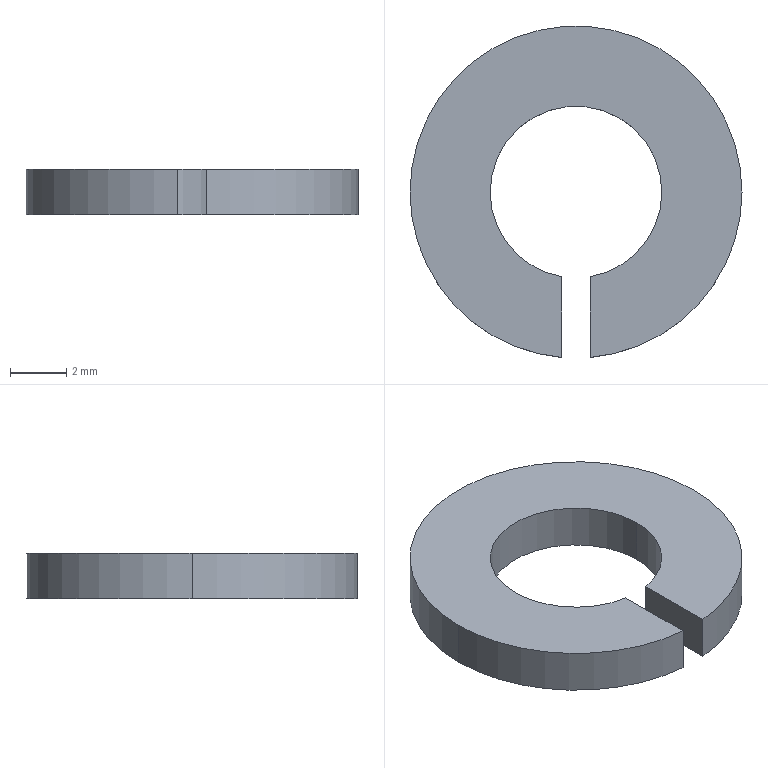Part | NX | features BREP 1 | 1 solid | 10 faces | box 11.8 x 11.779 x 1.6 mm | volume 123.644 mm3 | cylinder 6 | plane 4 | commonest cylinder face diameters 6.1 x3 11.8 x3
STEP:
#1=CARTESIAN_POINT('',(3.05,0.,1.6));
#2=VERTEX_POINT('',#1);
#3=CARTESIAN_POINT('',(0.5,-3.009,1.6));
#4=VERTEX_POINT('',#3);
#5=CARTESIAN_POINT('',(0.,0.,1.6));
#6=DIRECTION('',(0.,0.,-1.));
#7=DIRECTION('',(1.,0.,0.));
#8=AXIS2_PLACEMENT_3D('',#5,#6,#7);
#9=CIRCLE('',#8,3.05);
#10=EDGE_CURVE('',#2,#4,#9,.T.);
#11=ORIENTED_EDGE('',*,*,#10,.F.);
#12=CARTESIAN_POINT('',(3.05,0.,0.));
#13=VERTEX_POINT('',#12);
#14=CARTESIAN_POINT('',(3.05,0.,1.6));
#15=DIRECTION('',(0.,0.,-1.));
#16=VECTOR('',#15,1000.);
#17=LINE('',#14,#16);
#18=EDGE_CURVE('',#2,#13,#17,.T.);
#19=ORIENTED_EDGE('',*,*,#18,.T.);
#20=CARTESIAN_POINT('',(0.5,-3.009,0.));
#21=VERTEX_POINT('',#20);
#22=CARTESIAN_POINT('',(0.,0.,0.));
#23=DIRECTION('',(0.,0.,-1.));
#24=DIRECTION('',(1.,0.,0.));
#25=AXIS2_PLACEMENT_3D('',#22,#23,#24);
#26=CIRCLE('',#25,3.05);
#27=EDGE_CURVE('',#13,#21,#26,.T.);
#28=ORIENTED_EDGE('',*,*,#27,.T.);
#29=CARTESIAN_POINT('',(0.5,-3.009,1.6));
#30=DIRECTION('',(0.,0.,-1.));
#31=VECTOR('',#30,1000.);
#32=LINE('',#29,#31);
#33=EDGE_CURVE('',#4,#21,#32,.T.);
#34=ORIENTED_EDGE('',*,*,#33,.F.);
#35=EDGE_LOOP('',(#11,#19,#28,#34));
#36=FACE_BOUND('',#35,.T.);
#37=CARTESIAN_POINT('',(0.,0.,1.6));
#38=DIRECTION('',(0.,0.,-1.));
#39=DIRECTION('',(-1.,0.,0.));
#40=AXIS2_PLACEMENT_3D('',#37,#38,#39);
#41=CYLINDRICAL_SURFACE('',#40,3.05);
#42=ADVANCED_FACE('',(#36),#41,.F.);
#43=ORIENTED_EDGE('',*,*,#18,.F.);
#44=CARTESIAN_POINT('',(-3.05,0.,1.6));
#45=VERTEX_POINT('',#44);
#46=CARTESIAN_POINT('',(0.,0.,1.6));
#47=DIRECTION('',(0.,0.,-1.));
#48=DIRECTION('',(1.,0.,0.));
#49=AXIS2_PLACEMENT_3D('',#46,#47,#48);
#50=CIRCLE('',#49,3.05);
#51=EDGE_CURVE('',#45,#2,#50,.T.);
#52=ORIENTED_EDGE('',*,*,#51,.F.);
#53=CARTESIAN_POINT('',(-3.05,0.,0.));
#54=VERTEX_POINT('',#53);
#55=CARTESIAN_POINT('',(-3.05,0.,1.6));
#56=DIRECTION('',(0.,0.,-1.));
#57=VECTOR('',#56,1000.);
#58=LINE('',#55,#57);
#59=EDGE_CURVE('',#45,#54,#58,.T.);
#60=ORIENTED_EDGE('',*,*,#59,.T.);
#61=CARTESIAN_POINT('',(0.,0.,0.));
#62=DIRECTION('',(0.,0.,-1.));
#63=DIRECTION('',(1.,0.,0.));
#64=AXIS2_PLACEMENT_3D('',#61,#62,#63);
#65=CIRCLE('',#64,3.05);
#66=EDGE_CURVE('',#54,#13,#65,.T.);
#67=ORIENTED_EDGE('',*,*,#66,.T.);
#68=EDGE_LOOP('',(#43,#52,#60,#67));
#69=FACE_BOUND('',#68,.T.);
#70=CARTESIAN_POINT('',(0.,0.,1.6));
#71=DIRECTION('',(0.,0.,-1.));
#72=DIRECTION('',(-1.,0.,0.));
#73=AXIS2_PLACEMENT_3D('',#70,#71,#72);
#74=CYLINDRICAL_SURFACE('',#73,3.05);
#75=ADVANCED_FACE('',(#69),#74,.F.);
#76=CARTESIAN_POINT('',(5.9,0.,1.6));
#77=VERTEX_POINT('',#76);
#78=CARTESIAN_POINT('',(-5.9,0.,1.6));
#79=VERTEX_POINT('',#78);
#80=CARTESIAN_POINT('',(0.,0.,1.6));
#81=DIRECTION('',(0.,0.,1.));
#82=DIRECTION('',(1.,0.,0.));
#83=AXIS2_PLACEMENT_3D('',#80,#81,#82);
#84=CIRCLE('',#83,5.9);
#85=EDGE_CURVE('',#77,#79,#84,.T.);
#86=ORIENTED_EDGE('',*,*,#85,.F.);
#87=CARTESIAN_POINT('',(5.9,0.,0.));
#88=VERTEX_POINT('',#87);
#89=CARTESIAN_POINT('',(5.9,0.,1.6));
#90=DIRECTION('',(0.,0.,-1.));
#91=VECTOR('',#90,1000.);
#92=LINE('',#89,#91);
#93=EDGE_CURVE('',#77,#88,#92,.T.);
#94=ORIENTED_EDGE('',*,*,#93,.T.);
#95=CARTESIAN_POINT('',(-5.9,0.,0.));
#96=VERTEX_POINT('',#95);
#97=CARTESIAN_POINT('',(0.,0.,0.));
#98=DIRECTION('',(0.,0.,1.));
#99=DIRECTION('',(1.,0.,0.));
#100=AXIS2_PLACEMENT_3D('',#97,#98,#99);
#101=CIRCLE('',#100,5.9);
#102=EDGE_CURVE('',#88,#96,#101,.T.);
#103=ORIENTED_EDGE('',*,*,#102,.T.);
#104=CARTESIAN_POINT('',(-5.9,0.,1.6));
#105=DIRECTION('',(0.,0.,-1.));
#106=VECTOR('',#105,1000.);
#107=LINE('',#104,#106);
#108=EDGE_CURVE('',#79,#96,#107,.T.);
#109=ORIENTED_EDGE('',*,*,#108,.F.);
#110=EDGE_LOOP('',(#86,#94,#103,#109));
#111=FACE_BOUND('',#110,.T.);
#112=CARTESIAN_POINT('',(0.,0.,1.6));
#113=DIRECTION('',(0.,0.,-1.));
#114=DIRECTION('',(-1.,0.,0.));
#115=AXIS2_PLACEMENT_3D('',#112,#113,#114);
#116=CYLINDRICAL_SURFACE('',#115,5.9);
#117=ADVANCED_FACE('',(#111),#116,.T.);
#118=CARTESIAN_POINT('',(-0.5,-5.879,1.6));
#119=VERTEX_POINT('',#118);
#120=CARTESIAN_POINT('',(0.,0.,1.6));
#121=DIRECTION('',(0.,0.,1.));
#122=DIRECTION('',(1.,0.,0.));
#123=AXIS2_PLACEMENT_3D('',#120,#121,#122);
#124=CIRCLE('',#123,5.9);
#125=EDGE_CURVE('',#79,#119,#124,.T.);
#126=ORIENTED_EDGE('',*,*,#125,.F.);
#127=ORIENTED_EDGE('',*,*,#108,.T.);
#128=CARTESIAN_POINT('',(-0.5,-5.879,0.));
#129=VERTEX_POINT('',#128);
#130=CARTESIAN_POINT('',(0.,0.,0.));
#131=DIRECTION('',(0.,0.,1.));
#132=DIRECTION('',(1.,0.,0.));
#133=AXIS2_PLACEMENT_3D('',#130,#131,#132);
#134=CIRCLE('',#133,5.9);
#135=EDGE_CURVE('',#96,#129,#134,.T.);
#136=ORIENTED_EDGE('',*,*,#135,.T.);
#137=CARTESIAN_POINT('',(-0.5,-5.879,1.6));
#138=DIRECTION('',(0.,0.,-1.));
#139=VECTOR('',#138,1000.);
#140=LINE('',#137,#139);
#141=EDGE_CURVE('',#119,#129,#140,.T.);
#142=ORIENTED_EDGE('',*,*,#141,.F.);
#143=EDGE_LOOP('',(#126,#127,#136,#142));
#144=FACE_BOUND('',#143,.T.);
#145=CARTESIAN_POINT('',(0.,0.,1.6));
#146=DIRECTION('',(0.,0.,-1.));
#147=DIRECTION('',(-1.,0.,0.));
#148=AXIS2_PLACEMENT_3D('',#145,#146,#147);
#149=CYLINDRICAL_SURFACE('',#148,5.9);
#150=ADVANCED_FACE('',(#144),#149,.T.);
#151=ORIENTED_EDGE('',*,*,#93,.F.);
#152=CARTESIAN_POINT('',(0.5,-5.879,1.6));
#153=VERTEX_POINT('',#152);
#154=CARTESIAN_POINT('',(0.,0.,1.6));
#155=DIRECTION('',(0.,0.,1.));
#156=DIRECTION('',(1.,0.,0.));
#157=AXIS2_PLACEMENT_3D('',#154,#155,#156);
#158=CIRCLE('',#157,5.9);
#159=EDGE_CURVE('',#153,#77,#158,.T.);
#160=ORIENTED_EDGE('',*,*,#159,.F.);
#161=CARTESIAN_POINT('',(0.5,-5.879,0.));
#162=VERTEX_POINT('',#161);
#163=CARTESIAN_POINT('',(0.5,-5.879,1.6));
#164=DIRECTION('',(0.,0.,-1.));
#165=VECTOR('',#164,1000.);
#166=LINE('',#163,#165);
#167=EDGE_CURVE('',#153,#162,#166,.T.);
#168=ORIENTED_EDGE('',*,*,#167,.T.);
#169=CARTESIAN_POINT('',(0.,0.,0.));
#170=DIRECTION('',(0.,0.,1.));
#171=DIRECTION('',(1.,0.,0.));
#172=AXIS2_PLACEMENT_3D('',#169,#170,#171);
#173=CIRCLE('',#172,5.9);
#174=EDGE_CURVE('',#162,#88,#173,.T.);
#175=ORIENTED_EDGE('',*,*,#174,.T.);
#176=EDGE_LOOP('',(#151,#160,#168,#175));
#177=FACE_BOUND('',#176,.T.);
#178=CARTESIAN_POINT('',(0.,0.,1.6));
#179=DIRECTION('',(0.,0.,-1.));
#180=DIRECTION('',(-1.,0.,0.));
#181=AXIS2_PLACEMENT_3D('',#178,#179,#180);
#182=CYLINDRICAL_SURFACE('',#181,5.9);
#183=ADVANCED_FACE('',(#177),#182,.T.);
#184=CARTESIAN_POINT('',(-0.5,-3.009,0.));
#185=VERTEX_POINT('',#184);
#186=CARTESIAN_POINT('',(-0.5,-3.009,0.));
#187=DIRECTION('',(0.,1.,0.));
#188=VECTOR('',#187,1000.);
#189=LINE('',#186,#188);
#190=EDGE_CURVE('',#129,#185,#189,.T.);
#191=ORIENTED_EDGE('',*,*,#190,.T.);
#192=CARTESIAN_POINT('',(-0.5,-3.009,1.6));
#193=VERTEX_POINT('',#192);
#194=CARTESIAN_POINT('',(-0.5,-3.009,1.6));
#195=DIRECTION('',(0.,0.,-1.));
#196=VECTOR('',#195,1000.);
#197=LINE('',#194,#196);
#198=EDGE_CURVE('',#193,#185,#197,.T.);
#199=ORIENTED_EDGE('',*,*,#198,.F.);
#200=CARTESIAN_POINT('',(-0.5,-3.009,1.6));
#201=DIRECTION('',(0.,1.,0.));
#202=VECTOR('',#201,1000.);
#203=LINE('',#200,#202);
#204=EDGE_CURVE('',#119,#193,#203,.T.);
#205=ORIENTED_EDGE('',*,*,#204,.F.);
#206=ORIENTED_EDGE('',*,*,#141,.T.);
#207=EDGE_LOOP('',(#191,#199,#205,#206));
#208=FACE_BOUND('',#207,.T.);
#209=CARTESIAN_POINT('',(-0.5,-3.009,1.6));
#210=DIRECTION('',(-1.,0.,0.));
#211=DIRECTION('',(0.,1.,0.));
#212=AXIS2_PLACEMENT_3D('',#209,#210,#211);
#213=PLANE('',#212);
#214=ADVANCED_FACE('',(#208),#213,.F.);
#215=ORIENTED_EDGE('',*,*,#59,.F.);
#216=CARTESIAN_POINT('',(0.,0.,1.6));
#217=DIRECTION('',(0.,0.,-1.));
#218=DIRECTION('',(1.,0.,0.));
#219=AXIS2_PLACEMENT_3D('',#216,#217,#218);
#220=CIRCLE('',#219,3.05);
#221=EDGE_CURVE('',#193,#45,#220,.T.);
#222=ORIENTED_EDGE('',*,*,#221,.F.);
#223=ORIENTED_EDGE('',*,*,#198,.T.);
#224=CARTESIAN_POINT('',(0.,0.,0.));
#225=DIRECTION('',(0.,0.,-1.));
#226=DIRECTION('',(1.,0.,0.));
#227=AXIS2_PLACEMENT_3D('',#224,#225,#226);
#228=CIRCLE('',#227,3.05);
#229=EDGE_CURVE('',#185,#54,#228,.T.);
#230=ORIENTED_EDGE('',*,*,#229,.T.);
#231=EDGE_LOOP('',(#215,#222,#223,#230));
#232=FACE_BOUND('',#231,.T.);
#233=CARTESIAN_POINT('',(0.,0.,1.6));
#234=DIRECTION('',(0.,0.,-1.));
#235=DIRECTION('',(-1.,0.,0.));
#236=AXIS2_PLACEMENT_3D('',#233,#234,#235);
#237=CYLINDRICAL_SURFACE('',#236,3.05);
#238=ADVANCED_FACE('',(#232),#237,.F.);
#239=CARTESIAN_POINT('',(0.5,-3.009,0.));
#240=DIRECTION('',(0.,-1.,0.));
#241=VECTOR('',#240,1000.);
#242=LINE('',#239,#241);
#243=EDGE_CURVE('',#21,#162,#242,.T.);
#244=ORIENTED_EDGE('',*,*,#243,.T.);
#245=ORIENTED_EDGE('',*,*,#167,.F.);
#246=CARTESIAN_POINT('',(0.5,-3.009,1.6));
#247=DIRECTION('',(0.,-1.,0.));
#248=VECTOR('',#247,1000.);
#249=LINE('',#246,#248);
#250=EDGE_CURVE('',#4,#153,#249,.T.);
#251=ORIENTED_EDGE('',*,*,#250,.F.);
#252=ORIENTED_EDGE('',*,*,#33,.T.);
#253=EDGE_LOOP('',(#244,#245,#251,#252));
#254=FACE_BOUND('',#253,.T.);
#255=CARTESIAN_POINT('',(0.5,-3.009,1.6));
#256=DIRECTION('',(1.,0.,0.));
#257=DIRECTION('',(0.,1.,0.));
#258=AXIS2_PLACEMENT_3D('',#255,#256,#257);
#259=PLANE('',#258);
#260=ADVANCED_FACE('',(#254),#259,.F.);
#261=ORIENTED_EDGE('',*,*,#159,.T.);
#262=ORIENTED_EDGE('',*,*,#85,.T.);
#263=ORIENTED_EDGE('',*,*,#125,.T.);
#264=ORIENTED_EDGE('',*,*,#204,.T.);
#265=ORIENTED_EDGE('',*,*,#221,.T.);
#266=ORIENTED_EDGE('',*,*,#51,.T.);
#267=ORIENTED_EDGE('',*,*,#10,.T.);
#268=ORIENTED_EDGE('',*,*,#250,.T.);
#269=EDGE_LOOP('',(#261,#262,#263,#264,#265,#266,#267,#268));
#270=FACE_BOUND('',#269,.T.);
#271=CARTESIAN_POINT('',(0.,0.,1.6));
#272=DIRECTION('',(0.,0.,1.));
#273=DIRECTION('',(1.,0.,0.));
#274=AXIS2_PLACEMENT_3D('',#271,#272,#273);
#275=PLANE('',#274);
#276=ADVANCED_FACE('',(#270),#275,.T.);
#277=ORIENTED_EDGE('',*,*,#174,.F.);
#278=ORIENTED_EDGE('',*,*,#243,.F.);
#279=ORIENTED_EDGE('',*,*,#27,.F.);
#280=ORIENTED_EDGE('',*,*,#66,.F.);
#281=ORIENTED_EDGE('',*,*,#229,.F.);
#282=ORIENTED_EDGE('',*,*,#190,.F.);
#283=ORIENTED_EDGE('',*,*,#135,.F.);
#284=ORIENTED_EDGE('',*,*,#102,.F.);
#285=EDGE_LOOP('',(#277,#278,#279,#280,#281,#282,#283,#284));
#286=FACE_BOUND('',#285,.T.);
#287=CARTESIAN_POINT('',(0.,0.,0.));
#288=DIRECTION('',(0.,0.,1.));
#289=DIRECTION('',(1.,0.,0.));
#290=AXIS2_PLACEMENT_3D('',#287,#288,#289);
#291=PLANE('',#290);
#292=ADVANCED_FACE('',(#286),#291,.F.);
#293=CLOSED_SHELL('',(#42,#75,#117,#150,#183,#214,#238,#260,#276,#292));
#294=MANIFOLD_SOLID_BREP('',#293);
#295=(LENGTH_UNIT()NAMED_UNIT(*)SI_UNIT(.MILLI.,.METRE.));
#296=UNCERTAINTY_MEASURE_WITH_UNIT(LENGTH_MEASURE(0.00001),#295,'','');
#297=(NAMED_UNIT(*)PLANE_ANGLE_UNIT()SI_UNIT($,.RADIAN.));
#298=(NAMED_UNIT(*)SI_UNIT($,.STERADIAN.)SOLID_ANGLE_UNIT());
#299=(GEOMETRIC_REPRESENTATION_CONTEXT(3)GLOBAL_UNCERTAINTY_ASSIGNED_CONTEXT((#296))GLOBAL_UNIT_ASSIGNED_CONTEXT((#295,#297,#298))REPRESENTATION_CONTEXT('',''));
#300=ADVANCED_BREP_SHAPE_REPRESENTATION('',(#294),#299);